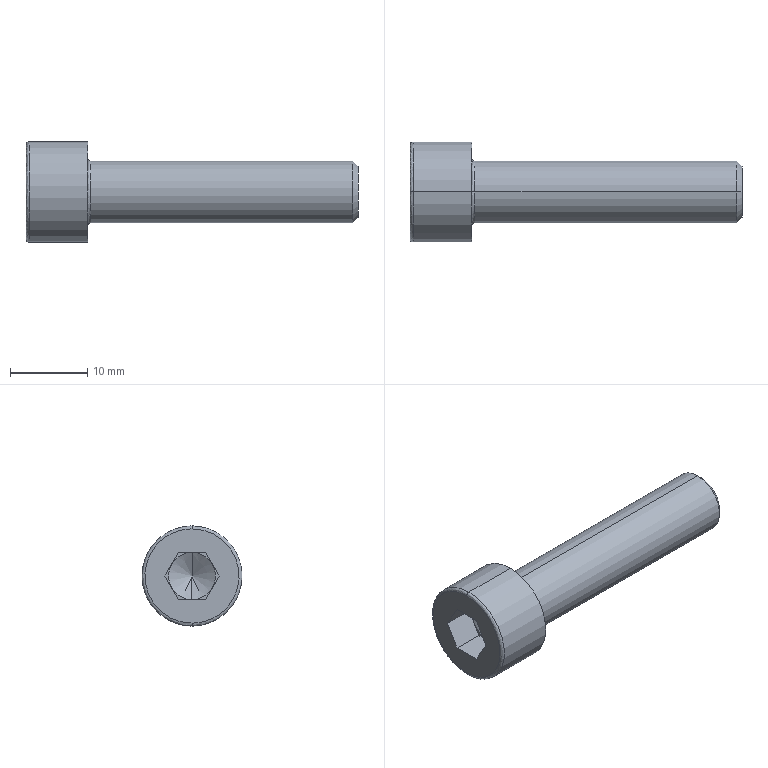Part | STEP file | 0229_311_M8x35 | 1 solid | 27 faces | box 43 x 13 x 13 mm | volume 2669 mm3 | plane 15 | spline 4 | cylinder 4 | cone 4 | commonest cylinder face diameters 8 x2 13 x2